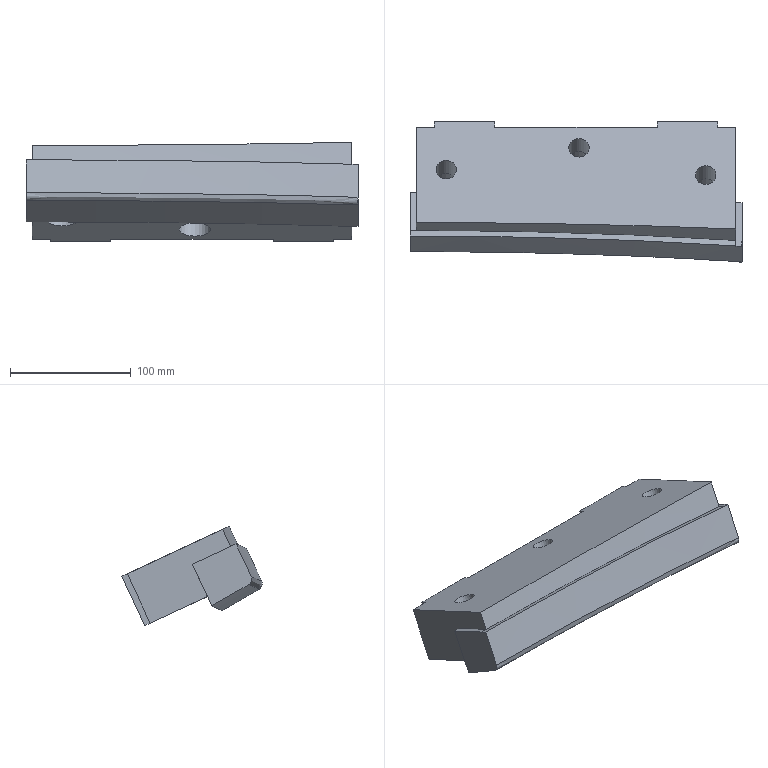Part | NX | features solid 2 | 1 solid | 33 faces | box 275 x 116.336 x 82.23 mm | volume 1182623 mm3 | plane 20 | spline 7 | cylinder 6 | commonest cylinder face diameters 17 x3 26 x3
STEP:
#1=CARTESIAN_POINT('',(270.,601.451,-143.671));
#2=VERTEX_POINT('',#1);
#3=CARTESIAN_POINT('',(255.,601.451,-143.671));
#4=VERTEX_POINT('',#3);
#5=CARTESIAN_POINT('',(575.,601.451,-143.671));
#6=DIRECTION('',(-1.,0.,0.));
#7=VECTOR('',#6,1000.);
#8=LINE('',#5,#7);
#9=EDGE_CURVE('',#2,#4,#8,.T.);
#10=ORIENTED_EDGE('',*,*,#9,.T.);
#11=CARTESIAN_POINT('',(255.,620.468,-102.887));
#12=VERTEX_POINT('',#11);
#13=CARTESIAN_POINT('',(255.,620.468,-102.887));
#14=DIRECTION('',(0.,-0.4226,-0.9063));
#15=VECTOR('',#14,1000.);
#16=LINE('',#13,#15);
#17=EDGE_CURVE('',#12,#4,#16,.T.);
#18=ORIENTED_EDGE('',*,*,#17,.F.);
#19=CARTESIAN_POINT('',(270.,620.468,-102.887));
#20=VERTEX_POINT('',#19);
#21=CARTESIAN_POINT('',(575.,620.468,-102.887));
#22=DIRECTION('',(1.,0.,0.));
#23=VECTOR('',#22,1000.);
#24=LINE('',#21,#23);
#25=EDGE_CURVE('',#20,#12,#24,.F.);
#26=ORIENTED_EDGE('',*,*,#25,.F.);
#27=CARTESIAN_POINT('',(270.,624.528,-94.181));
#28=DIRECTION('',(0.,-0.4226,-0.9063));
#29=VECTOR('',#28,1000.);
#30=LINE('',#27,#29);
#31=EDGE_CURVE('',#2,#20,#30,.F.);
#32=ORIENTED_EDGE('',*,*,#31,.F.);
#33=EDGE_LOOP('',(#10,#18,#26,#32));
#34=FACE_BOUND('',#33,.T.);
#35=CARTESIAN_POINT('',(575.,624.528,-94.181));
#36=DIRECTION('',(0.,-0.9063,0.4226));
#37=DIRECTION('',(0.,-0.4226,-0.9063));
#38=AXIS2_PLACEMENT_3D('',#35,#36,#37);
#39=PLANE('',#38);
#40=ADVANCED_FACE('',(#34),#39,.F.);
#41=CARTESIAN_POINT('',(205.,620.468,-102.887));
#42=VERTEX_POINT('',#41);
#43=CARTESIAN_POINT('',(70.,620.468,-102.887));
#44=VERTEX_POINT('',#43);
#45=CARTESIAN_POINT('',(575.,620.468,-102.887));
#46=DIRECTION('',(1.,0.,0.));
#47=VECTOR('',#46,1000.);
#48=LINE('',#45,#47);
#49=EDGE_CURVE('',#42,#44,#48,.F.);
#50=ORIENTED_EDGE('',*,*,#49,.F.);
#51=CARTESIAN_POINT('',(205.,601.451,-143.671));
#52=VERTEX_POINT('',#51);
#53=CARTESIAN_POINT('',(205.,620.468,-102.887));
#54=DIRECTION('',(0.,-0.4226,-0.9063));
#55=VECTOR('',#54,1000.);
#56=LINE('',#53,#55);
#57=EDGE_CURVE('',#42,#52,#56,.T.);
#58=ORIENTED_EDGE('',*,*,#57,.T.);
#59=CARTESIAN_POINT('',(70.,601.451,-143.671));
#60=VERTEX_POINT('',#59);
#61=CARTESIAN_POINT('',(575.,601.451,-143.671));
#62=DIRECTION('',(-1.,0.,0.));
#63=VECTOR('',#62,1000.);
#64=LINE('',#61,#63);
#65=EDGE_CURVE('',#52,#60,#64,.T.);
#66=ORIENTED_EDGE('',*,*,#65,.T.);
#67=CARTESIAN_POINT('',(70.,620.468,-102.887));
#68=DIRECTION('',(0.,-0.4226,-0.9063));
#69=VECTOR('',#68,1000.);
#70=LINE('',#67,#69);
#71=EDGE_CURVE('',#44,#60,#70,.T.);
#72=ORIENTED_EDGE('',*,*,#71,.F.);
#73=EDGE_LOOP('',(#50,#58,#66,#72));
#74=FACE_BOUND('',#73,.T.);
#75=CARTESIAN_POINT('',(575.,624.528,-94.181));
#76=DIRECTION('',(0.,-0.9063,0.4226));
#77=DIRECTION('',(0.,-0.4226,-0.9063));
#78=AXIS2_PLACEMENT_3D('',#75,#76,#77);
#79=PLANE('',#78);
#80=ADVANCED_FACE('',(#74),#79,.F.);
#81=CARTESIAN_POINT('',(20.,620.468,-102.887));
#82=VERTEX_POINT('',#81);
#83=CARTESIAN_POINT('',(5.,620.468,-102.887));
#84=VERTEX_POINT('',#83);
#85=CARTESIAN_POINT('',(575.,620.468,-102.887));
#86=DIRECTION('',(1.,0.,0.));
#87=VECTOR('',#86,1000.);
#88=LINE('',#85,#87);
#89=EDGE_CURVE('',#82,#84,#88,.F.);
#90=ORIENTED_EDGE('',*,*,#89,.F.);
#91=CARTESIAN_POINT('',(20.,601.451,-143.671));
#92=VERTEX_POINT('',#91);
#93=CARTESIAN_POINT('',(20.,620.468,-102.887));
#94=DIRECTION('',(0.,-0.4226,-0.9063));
#95=VECTOR('',#94,1000.);
#96=LINE('',#93,#95);
#97=EDGE_CURVE('',#82,#92,#96,.T.);
#98=ORIENTED_EDGE('',*,*,#97,.T.);
#99=CARTESIAN_POINT('',(5.,601.451,-143.671));
#100=VERTEX_POINT('',#99);
#101=CARTESIAN_POINT('',(575.,601.451,-143.671));
#102=DIRECTION('',(-1.,0.,0.));
#103=VECTOR('',#102,1000.);
#104=LINE('',#101,#103);
#105=EDGE_CURVE('',#92,#100,#104,.T.);
#106=ORIENTED_EDGE('',*,*,#105,.T.);
#107=CARTESIAN_POINT('',(5.,624.528,-94.181));
#108=DIRECTION('',(0.,0.4226,0.9063));
#109=VECTOR('',#108,1000.);
#110=LINE('',#107,#109);
#111=EDGE_CURVE('',#84,#100,#110,.F.);
#112=ORIENTED_EDGE('',*,*,#111,.F.);
#113=EDGE_LOOP('',(#90,#98,#106,#112));
#114=FACE_BOUND('',#113,.T.);
#115=CARTESIAN_POINT('',(575.,624.528,-94.181));
#116=DIRECTION('',(0.,-0.9063,0.4226));
#117=DIRECTION('',(0.,-0.4226,-0.9063));
#118=AXIS2_PLACEMENT_3D('',#115,#116,#117);
#119=PLANE('',#118);
#120=ADVANCED_FACE('',(#114),#119,.F.);
#121=CARTESIAN_POINT('',(275.,521.829,-81.79));
#122=VERTEX_POINT('',#121);
#123=CARTESIAN_POINT('',(275.,526.352,-83.884));
#124=VERTEX_POINT('',#123);
#125=CARTESIAN_POINT('',(275.,521.829,-81.79));
#126=CARTESIAN_POINT('',(275.,523.337,-82.488));
#127=CARTESIAN_POINT('',(275.,524.845,-83.186));
#128=CARTESIAN_POINT('',(275.,526.352,-83.884));
#129=B_SPLINE_CURVE_WITH_KNOTS('',3,(#125,#126,#127,#128),.UNSPECIFIED.,.F.,.F.,(4,4),(0.001536,0.00652),.UNSPECIFIED.);
#130=EDGE_CURVE('',#122,#124,#129,.T.);
#131=ORIENTED_EDGE('',*,*,#130,.T.);
#132=CARTESIAN_POINT('',(274.761,521.845,-81.782));
#133=VERTEX_POINT('',#132);
#134=CARTESIAN_POINT('',(275.,526.352,-83.884));
#135=CARTESIAN_POINT('',(274.92,524.85,-83.183));
#136=CARTESIAN_POINT('',(274.84,523.348,-82.483));
#137=CARTESIAN_POINT('',(274.761,521.845,-81.782));
#138=B_SPLINE_CURVE_WITH_KNOTS('',3,(#134,#135,#136,#137),.UNSPECIFIED.,.F.,.F.,(4,4),(0.00005195,0.005031),.UNSPECIFIED.);
#139=EDGE_CURVE('',#124,#133,#138,.T.);
#140=ORIENTED_EDGE('',*,*,#139,.T.);
#141=CARTESIAN_POINT('',(275.,521.829,-81.79));
#142=CARTESIAN_POINT('',(274.92,521.835,-81.787));
#143=CARTESIAN_POINT('',(274.84,521.84,-81.785));
#144=CARTESIAN_POINT('',(274.761,521.845,-81.782));
#145=B_SPLINE_CURVE_WITH_KNOTS('',3,(#141,#142,#143,#144),.UNSPECIFIED.,.F.,.F.,(4,4),(0.2861,0.2864),.UNSPECIFIED.);
#146=EDGE_CURVE('',#122,#133,#145,.T.);
#147=ORIENTED_EDGE('',*,*,#146,.F.);
#148=EDGE_LOOP('',(#131,#140,#147));
#149=FACE_BOUND('',#148,.T.);
#150=CARTESIAN_POINT('',(275.243,526.363,-83.904));
#151=CARTESIAN_POINT('',(275.162,526.369,-83.901));
#152=CARTESIAN_POINT('',(275.082,526.374,-83.899));
#153=CARTESIAN_POINT('',(275.001,526.379,-83.896));
#154=CARTESIAN_POINT('',(275.242,526.355,-83.9));
#155=CARTESIAN_POINT('',(275.162,526.361,-83.898));
#156=CARTESIAN_POINT('',(275.081,526.366,-83.895));
#157=CARTESIAN_POINT('',(275.001,526.372,-83.893));
#158=CARTESIAN_POINT('',(275.,521.802,-81.777));
#159=CARTESIAN_POINT('',(274.92,521.808,-81.775));
#160=CARTESIAN_POINT('',(274.839,521.813,-81.772));
#161=CARTESIAN_POINT('',(274.759,521.818,-81.77));
#162=B_SPLINE_SURFACE_WITH_KNOTS('',1,3,((#150,#151,#152,#153),(#154,#155,#156,#157),(#158,#159,#160,#161)),.RULED_SURF.,.F.,.F.,.F.,(2,1,2),(4,4),(-0.0008614,0.,0.503),(0.2539,0.2541),.PIECEWISE_BEZIER_KNOTS.);
#163=ADVANCED_FACE('',(#149),#162,.F.);
#164=CARTESIAN_POINT('',(0.,566.489,-94.945));
#165=VERTEX_POINT('',#164);
#166=CARTESIAN_POINT('',(0.,534.859,-80.196));
#167=VERTEX_POINT('',#166);
#168=CARTESIAN_POINT('',(0.,-410.961,360.847));
#169=DIRECTION('',(0.,-0.9063,0.4226));
#170=VECTOR('',#169,1000.);
#171=LINE('',#168,#170);
#172=EDGE_CURVE('',#165,#167,#171,.T.);
#173=ORIENTED_EDGE('',*,*,#172,.F.);
#174=CARTESIAN_POINT('',(0.1494,550.411,-129.426));
#175=VERTEX_POINT('',#174);
#176=CARTESIAN_POINT('',(0.,541.565,-148.396));
#177=DIRECTION('',(0.,0.4226,0.9063));
#178=VECTOR('',#177,1000.);
#179=LINE('',#176,#178);
#180=EDGE_CURVE('',#175,#165,#179,.T.);
#181=ORIENTED_EDGE('',*,*,#180,.F.);
#182=CARTESIAN_POINT('',(0.1308,519.6,-111.637));
#183=VERTEX_POINT('',#182);
#184=CARTESIAN_POINT('',(0.,519.507,-111.584));
#185=CARTESIAN_POINT('',(0.,529.898,-117.583));
#186=CARTESIAN_POINT('',(0.,540.289,-123.583));
#187=CARTESIAN_POINT('',(0.,550.68,-129.582));
#188=B_SPLINE_CURVE_WITH_KNOTS('',3,(#184,#185,#186,#187),.UNSPECIFIED.,.F.,.F.,(4,4),(0.,1.),.UNSPECIFIED.);
#189=EDGE_CURVE('',#183,#175,#188,.T.);
#190=ORIENTED_EDGE('',*,*,#189,.F.);
#191=CARTESIAN_POINT('',(0.1262,517.66,-105.247));
#192=VERTEX_POINT('',#191);
#193=CARTESIAN_POINT('',(0.,517.66,-105.248));
#194=CARTESIAN_POINT('',(0.,517.387,-105.835));
#195=CARTESIAN_POINT('',(0.,517.07,-107.013));
#196=CARTESIAN_POINT('',(0.,517.318,-108.896));
#197=CARTESIAN_POINT('',(0.,518.194,-110.583));
#198=CARTESIAN_POINT('',(0.,519.13,-111.367));
#199=CARTESIAN_POINT('',(0.,519.692,-111.691));
#200=B_SPLINE_CURVE_WITH_KNOTS('',3,(#193,#194,#195,#196,#197,#198,#199),.UNSPECIFIED.,.F.,.F.,(4,1,1,1,4),(0.,0.25,0.5,0.75,1.),.UNSPECIFIED.);
#201=EDGE_CURVE('',#192,#183,#200,.T.);
#202=ORIENTED_EDGE('',*,*,#201,.F.);
#203=CARTESIAN_POINT('',(0.,530.327,-78.083));
#204=VERTEX_POINT('',#203);
#205=CARTESIAN_POINT('',(0.,514.598,-111.815));
#206=DIRECTION('',(0.,0.4226,0.9063));
#207=VECTOR('',#206,1000.);
#208=LINE('',#205,#207);
#209=EDGE_CURVE('',#192,#204,#208,.T.);
#210=ORIENTED_EDGE('',*,*,#209,.T.);
#211=CARTESIAN_POINT('',(0.,530.327,-78.083));
#212=CARTESIAN_POINT('',(0.,531.838,-78.787));
#213=CARTESIAN_POINT('',(0.,533.349,-79.492));
#214=CARTESIAN_POINT('',(0.,534.859,-80.196));
#215=B_SPLINE_CURVE_WITH_KNOTS('',3,(#211,#212,#213,#214),.UNSPECIFIED.,.F.,.F.,(4,4),(0.001534,0.006534),.UNSPECIFIED.);
#216=EDGE_CURVE('',#204,#167,#215,.T.);
#217=ORIENTED_EDGE('',*,*,#216,.T.);
#218=EDGE_LOOP('',(#173,#181,#190,#202,#210,#217));
#219=FACE_BOUND('',#218,.T.);
#220=CARTESIAN_POINT('',(0.,-402.415,379.173));
#221=DIRECTION('',(-1.,0.,0.));
#222=DIRECTION('',(0.,-1.,0.));
#223=AXIS2_PLACEMENT_3D('',#220,#221,#222);
#224=PLANE('',#223);
#225=ADVANCED_FACE('',(#219),#224,.T.);
#226=CARTESIAN_POINT('',(275.,541.913,-133.245));
#227=VERTEX_POINT('',#226);
#228=CARTESIAN_POINT('',(275.,558.04,-98.66));
#229=VERTEX_POINT('',#228);
#230=CARTESIAN_POINT('',(275.,536.047,-145.824));
#231=DIRECTION('',(0.,0.4226,0.9063));
#232=VECTOR('',#231,1000.);
#233=LINE('',#230,#232);
#234=EDGE_CURVE('',#227,#229,#233,.T.);
#235=ORIENTED_EDGE('',*,*,#234,.T.);
#236=CARTESIAN_POINT('',(275.,-413.893,354.56));
#237=DIRECTION('',(0.,-0.9063,0.4226));
#238=VECTOR('',#237,1000.);
#239=LINE('',#236,#238);
#240=EDGE_CURVE('',#229,#124,#239,.T.);
#241=ORIENTED_EDGE('',*,*,#240,.T.);
#242=ORIENTED_EDGE('',*,*,#130,.F.);
#243=CARTESIAN_POINT('',(275.,509.13,-109.022));
#244=VERTEX_POINT('',#243);
#245=CARTESIAN_POINT('',(275.,509.037,-109.222));
#246=DIRECTION('',(0.,0.4226,0.9063));
#247=VECTOR('',#246,1000.);
#248=LINE('',#245,#247);
#249=EDGE_CURVE('',#244,#122,#248,.T.);
#250=ORIENTED_EDGE('',*,*,#249,.F.);
#251=CARTESIAN_POINT('',(275.,511.154,-115.455));
#252=VERTEX_POINT('',#251);
#253=CARTESIAN_POINT('',(275.,509.13,-109.022));
#254=CARTESIAN_POINT('',(275.,508.604,-110.151));
#255=CARTESIAN_POINT('',(275.,508.441,-112.771));
#256=CARTESIAN_POINT('',(275.,510.076,-114.832));
#257=CARTESIAN_POINT('',(275.,511.154,-115.455));
#258=B_SPLINE_CURVE_WITH_KNOTS('',3,(#253,#254,#255,#256,#257),.UNSPECIFIED.,.F.,.F.,(4,1,4),(0.,0.003682,0.007364),.UNSPECIFIED.);
#259=EDGE_CURVE('',#244,#252,#258,.T.);
#260=ORIENTED_EDGE('',*,*,#259,.T.);
#261=CARTESIAN_POINT('',(275.,511.154,-115.455));
#262=CARTESIAN_POINT('',(275.,521.407,-121.385));
#263=CARTESIAN_POINT('',(275.,531.66,-127.315));
#264=CARTESIAN_POINT('',(275.,541.913,-133.245));
#265=B_SPLINE_CURVE_WITH_KNOTS('',3,(#261,#262,#263,#264),.UNSPECIFIED.,.F.,.F.,(4,4),(0.0002564,0.03579),.UNSPECIFIED.);
#266=EDGE_CURVE('',#252,#227,#265,.T.);
#267=ORIENTED_EDGE('',*,*,#266,.T.);
#268=EDGE_LOOP('',(#235,#241,#242,#250,#260,#267));
#269=FACE_BOUND('',#268,.T.);
#270=CARTESIAN_POINT('',(275.,-402.415,379.173));
#271=DIRECTION('',(-1.,0.,0.));
#272=DIRECTION('',(0.,-1.,0.));
#273=AXIS2_PLACEMENT_3D('',#270,#271,#272);
#274=PLANE('',#273);
#275=ADVANCED_FACE('',(#269),#274,.F.);
#276=CARTESIAN_POINT('',(30.,593.005,-90.081));
#277=VERTEX_POINT('',#276);
#278=CARTESIAN_POINT('',(30.,585.302,-86.488));
#279=DIRECTION('',(0.,-0.4226,-0.9063));
#280=DIRECTION('',(0.,0.9063,-0.4226));
#281=AXIS2_PLACEMENT_3D('',#278,#279,#280);
#282=CIRCLE('',#281,8.5);
#283=EDGE_CURVE('',#277,#277,#282,.T.);
#284=ORIENTED_EDGE('',*,*,#283,.T.);
#285=EDGE_LOOP('',(#284));
#286=FACE_BOUND('',#285,.T.);
#287=CARTESIAN_POINT('',(140.,611.132,-98.533));
#288=VERTEX_POINT('',#287);
#289=CARTESIAN_POINT('',(140.,603.428,-94.941));
#290=DIRECTION('',(0.,-0.4226,-0.9063));
#291=DIRECTION('',(0.,0.9063,-0.4226));
#292=AXIS2_PLACEMENT_3D('',#289,#290,#291);
#293=CIRCLE('',#292,8.5);
#294=EDGE_CURVE('',#288,#288,#293,.T.);
#295=ORIENTED_EDGE('',*,*,#294,.T.);
#296=EDGE_LOOP('',(#295));
#297=FACE_BOUND('',#296,.T.);
#298=CARTESIAN_POINT('',(245.,588.474,-87.968));
#299=VERTEX_POINT('',#298);
#300=CARTESIAN_POINT('',(245.,580.77,-84.375));
#301=DIRECTION('',(0.,-0.4226,-0.9063));
#302=DIRECTION('',(0.,0.9063,-0.4226));
#303=AXIS2_PLACEMENT_3D('',#300,#301,#302);
#304=CIRCLE('',#303,8.5);
#305=EDGE_CURVE('',#299,#299,#304,.T.);
#306=ORIENTED_EDGE('',*,*,#305,.T.);
#307=EDGE_LOOP('',(#306));
#308=FACE_BOUND('',#307,.T.);
#309=ORIENTED_EDGE('',*,*,#25,.T.);
#310=CARTESIAN_POINT('',(255.,625.,-105.));
#311=VERTEX_POINT('',#310);
#312=CARTESIAN_POINT('',(255.,620.468,-102.887));
#313=DIRECTION('',(0.,-0.9063,0.4226));
#314=VECTOR('',#313,1000.);
#315=LINE('',#312,#314);
#316=EDGE_CURVE('',#12,#311,#315,.F.);
#317=ORIENTED_EDGE('',*,*,#316,.T.);
#318=CARTESIAN_POINT('',(205.,625.,-105.));
#319=VERTEX_POINT('',#318);
#320=CARTESIAN_POINT('',(255.,625.,-105.));
#321=DIRECTION('',(1.,0.,0.));
#322=VECTOR('',#321,1000.);
#323=LINE('',#320,#322);
#324=EDGE_CURVE('',#311,#319,#323,.F.);
#325=ORIENTED_EDGE('',*,*,#324,.T.);
#326=CARTESIAN_POINT('',(205.,620.468,-102.887));
#327=DIRECTION('',(0.,-0.9063,0.4226));
#328=VECTOR('',#327,1000.);
#329=LINE('',#326,#328);
#330=EDGE_CURVE('',#42,#319,#329,.F.);
#331=ORIENTED_EDGE('',*,*,#330,.F.);
#332=ORIENTED_EDGE('',*,*,#49,.T.);
#333=CARTESIAN_POINT('',(70.,625.,-105.));
#334=VERTEX_POINT('',#333);
#335=CARTESIAN_POINT('',(70.,620.468,-102.887));
#336=DIRECTION('',(0.,-0.9063,0.4226));
#337=VECTOR('',#336,1000.);
#338=LINE('',#335,#337);
#339=EDGE_CURVE('',#44,#334,#338,.F.);
#340=ORIENTED_EDGE('',*,*,#339,.T.);
#341=CARTESIAN_POINT('',(20.,625.,-105.));
#342=VERTEX_POINT('',#341);
#343=CARTESIAN_POINT('',(20.,625.,-105.));
#344=DIRECTION('',(1.,0.,0.));
#345=VECTOR('',#344,1000.);
#346=LINE('',#343,#345);
#347=EDGE_CURVE('',#342,#334,#346,.T.);
#348=ORIENTED_EDGE('',*,*,#347,.F.);
#349=CARTESIAN_POINT('',(20.,620.468,-102.887));
#350=DIRECTION('',(0.,-0.9063,0.4226));
#351=VECTOR('',#350,1000.);
#352=LINE('',#349,#351);
#353=EDGE_CURVE('',#82,#342,#352,.F.);
#354=ORIENTED_EDGE('',*,*,#353,.F.);
#355=ORIENTED_EDGE('',*,*,#89,.T.);
#356=CARTESIAN_POINT('',(5.,541.457,-66.043));
#357=VERTEX_POINT('',#356);
#358=CARTESIAN_POINT('',(5.,568.557,-78.68));
#359=DIRECTION('',(0.,-0.9063,0.4226));
#360=VECTOR('',#359,1000.);
#361=LINE('',#358,#360);
#362=EDGE_CURVE('',#84,#357,#361,.T.);
#363=ORIENTED_EDGE('',*,*,#362,.T.);
#364=CARTESIAN_POINT('',(270.,536.118,-63.554));
#365=VERTEX_POINT('',#364);
#366=CARTESIAN_POINT('',(5.,541.457,-66.043));
#367=CARTESIAN_POINT('',(49.188,541.427,-66.029));
#368=CARTESIAN_POINT('',(137.544,540.561,-65.626));
#369=CARTESIAN_POINT('',(225.858,537.997,-64.43));
#370=CARTESIAN_POINT('',(270.,536.118,-63.554));
#371=B_SPLINE_CURVE_WITH_KNOTS('',3,(#366,#367,#368,#369,#370),.UNSPECIFIED.,.F.,.F.,(4,1,4),(0.,0.1325,0.2651),.UNSPECIFIED.);
#372=EDGE_CURVE('',#357,#365,#371,.T.);
#373=ORIENTED_EDGE('',*,*,#372,.T.);
#374=CARTESIAN_POINT('',(270.,568.557,-78.68));
#375=DIRECTION('',(0.,0.9063,-0.4226));
#376=VECTOR('',#375,1000.);
#377=LINE('',#374,#376);
#378=EDGE_CURVE('',#365,#20,#377,.T.);
#379=ORIENTED_EDGE('',*,*,#378,.T.);
#380=EDGE_LOOP('',(#309,#317,#325,#331,#332,#340,#348,#354,#355,#363,#373,#379));
#381=FACE_BOUND('',#380,.T.);
#382=CARTESIAN_POINT('',(0.0001507,568.557,-78.68));
#383=DIRECTION('',(0.,-0.4226,-0.9063));
#384=DIRECTION('',(0.,0.9063,-0.4226));
#385=AXIS2_PLACEMENT_3D('',#382,#383,#384);
#386=PLANE('',#385);
#387=ADVANCED_FACE('',(#286,#297,#308,#381),#386,.F.);
#388=CARTESIAN_POINT('',(275.,541.913,-133.245));
#389=CARTESIAN_POINT('',(252.161,543.463,-132.522));
#390=CARTESIAN_POINT('',(206.445,546.02,-131.369));
#391=CARTESIAN_POINT('',(137.772,548.579,-130.204));
#392=CARTESIAN_POINT('',(69.042,550.086,-129.551));
#393=CARTESIAN_POINT('',(23.212,550.391,-129.464));
#394=CARTESIAN_POINT('',(0.2987,550.41,-129.427));
#395=B_SPLINE_CURVE_WITH_KNOTS('',3,(#388,#389,#390,#391,#392,#393,#394),.UNSPECIFIED.,.F.,.F.,(4,1,1,1,4),(0.3277,0.3968,0.4659,0.535,0.6041),.UNSPECIFIED.);
#396=EDGE_CURVE('',#227,#175,#395,.T.);
#397=ORIENTED_EDGE('',*,*,#396,.T.);
#398=ORIENTED_EDGE('',*,*,#180,.T.);
#399=CARTESIAN_POINT('',(5.,566.487,-94.945));
#400=VERTEX_POINT('',#399);
#401=CARTESIAN_POINT('',(5.,566.487,-94.945));
#402=CARTESIAN_POINT('',(3.333,566.489,-94.945));
#403=CARTESIAN_POINT('',(1.667,566.489,-94.945));
#404=CARTESIAN_POINT('',(0.,566.489,-94.945));
#405=B_SPLINE_CURVE_WITH_KNOTS('',3,(#401,#402,#403,#404),.UNSPECIFIED.,.F.,.F.,(4,4),(0.,0.005),.UNSPECIFIED.);
#406=EDGE_CURVE('',#400,#165,#405,.T.);
#407=ORIENTED_EDGE('',*,*,#406,.F.);
#408=CARTESIAN_POINT('',(5.,554.069,-121.576));
#409=VERTEX_POINT('',#408);
#410=CARTESIAN_POINT('',(5.,587.618,-49.629));
#411=DIRECTION('',(0.,0.4226,0.9063));
#412=VECTOR('',#411,1000.);
#413=LINE('',#410,#412);
#414=EDGE_CURVE('',#409,#400,#413,.T.);
#415=ORIENTED_EDGE('',*,*,#414,.F.);
#416=CARTESIAN_POINT('',(270.,548.769,-119.105));
#417=VERTEX_POINT('',#416);
#418=CARTESIAN_POINT('',(270.,548.769,-119.105));
#419=CARTESIAN_POINT('',(225.874,550.647,-119.981));
#420=CARTESIAN_POINT('',(137.542,553.172,-121.158));
#421=CARTESIAN_POINT('',(49.177,554.039,-121.562));
#422=CARTESIAN_POINT('',(5.,554.069,-121.576));
#423=B_SPLINE_CURVE_WITH_KNOTS('',3,(#418,#419,#420,#421,#422),.UNSPECIFIED.,.F.,.F.,(4,1,4),(0.3304,0.4638,0.5972),.UNSPECIFIED.);
#424=EDGE_CURVE('',#409,#417,#423,.F.);
#425=ORIENTED_EDGE('',*,*,#424,.T.);
#426=CARTESIAN_POINT('',(270.,558.255,-98.76));
#427=VERTEX_POINT('',#426);
#428=CARTESIAN_POINT('',(270.,579.386,-53.445));
#429=DIRECTION('',(0.,0.4226,0.9063));
#430=VECTOR('',#429,1000.);
#431=LINE('',#428,#430);
#432=EDGE_CURVE('',#417,#427,#431,.T.);
#433=ORIENTED_EDGE('',*,*,#432,.T.);
#434=CARTESIAN_POINT('',(275.,558.04,-98.66));
#435=CARTESIAN_POINT('',(273.333,558.113,-98.694));
#436=CARTESIAN_POINT('',(271.667,558.185,-98.727));
#437=CARTESIAN_POINT('',(270.,558.255,-98.76));
#438=B_SPLINE_CURVE_WITH_KNOTS('',3,(#434,#435,#436,#437),.UNSPECIFIED.,.F.,.F.,(4,4),(0.,0.005006),.UNSPECIFIED.);
#439=EDGE_CURVE('',#229,#427,#438,.T.);
#440=ORIENTED_EDGE('',*,*,#439,.F.);
#441=ORIENTED_EDGE('',*,*,#234,.F.);
#442=EDGE_LOOP('',(#397,#398,#407,#415,#425,#433,#440,#441));
#443=FACE_BOUND('',#442,.T.);
#444=CARTESIAN_POINT('',(275.,541.798,-133.491));
#445=CARTESIAN_POINT('',(275.,560.972,-92.373));
#446=CARTESIAN_POINT('',(229.14,543.799,-134.424));
#447=CARTESIAN_POINT('',(229.14,562.973,-93.306));
#448=CARTESIAN_POINT('',(137.488,546.449,-135.659));
#449=CARTESIAN_POINT('',(137.488,565.622,-94.541));
#450=CARTESIAN_POINT('',(45.83,547.315,-136.063));
#451=CARTESIAN_POINT('',(45.83,566.489,-94.945));
#452=CARTESIAN_POINT('',(0.,547.316,-136.063));
#453=CARTESIAN_POINT('',(0.,566.489,-94.945));
#454=B_SPLINE_SURFACE_WITH_KNOTS('',3,1,((#444,#445),(#446,#447),(#448,#449),(#450,#451),(#452,#453)),.SURF_OF_LINEAR_EXTRUSION.,.F.,.F.,.F.,(4,1,4),(2,2),(0.259,0.3795,0.5),(0.,1.),.UNSPECIFIED.);
#455=ADVANCED_FACE('',(#443),#454,.T.);
#456=ORIENTED_EDGE('',*,*,#266,.F.);
#457=CARTESIAN_POINT('',(275.,511.154,-115.455));
#458=CARTESIAN_POINT('',(252.136,512.708,-114.74));
#459=CARTESIAN_POINT('',(206.371,515.266,-113.597));
#460=CARTESIAN_POINT('',(137.64,517.859,-112.459));
#461=CARTESIAN_POINT('',(68.827,519.374,-111.816));
#462=CARTESIAN_POINT('',(22.943,519.674,-111.729));
#463=CARTESIAN_POINT('',(0.00009814,519.692,-111.691));
#464=B_SPLINE_CURVE_WITH_KNOTS('',3,(#457,#458,#459,#460,#461,#462,#463),.UNSPECIFIED.,.F.,.F.,(4,1,1,1,4),(0.08355,0.1523,0.2211,0.2899,0.3587),.UNSPECIFIED.);
#465=EDGE_CURVE('',#252,#183,#464,.T.);
#466=ORIENTED_EDGE('',*,*,#465,.T.);
#467=ORIENTED_EDGE('',*,*,#189,.T.);
#468=ORIENTED_EDGE('',*,*,#396,.F.);
#469=EDGE_LOOP('',(#456,#466,#467,#468));
#470=FACE_BOUND('',#469,.T.);
#471=CARTESIAN_POINT('',(277.219,510.812,-115.416));
#472=CARTESIAN_POINT('',(276.64,541.986,-133.405));
#473=CARTESIAN_POINT('',(264.567,511.676,-115.01));
#474=CARTESIAN_POINT('',(264.035,542.849,-133.001));
#475=CARTESIAN_POINT('',(250.894,512.514,-114.625));
#476=CARTESIAN_POINT('',(250.405,543.687,-132.617));
#477=CARTESIAN_POINT('',(218.319,514.321,-113.806));
#478=CARTESIAN_POINT('',(217.92,545.495,-131.799));
#479=CARTESIAN_POINT('',(197.638,515.298,-113.372));
#480=CARTESIAN_POINT('',(197.285,546.471,-131.367));
#481=CARTESIAN_POINT('',(158.795,516.84,-112.697));
#482=CARTESIAN_POINT('',(158.522,548.013,-130.693));
#483=CARTESIAN_POINT('',(138.351,517.497,-112.414));
#484=CARTESIAN_POINT('',(138.119,548.671,-130.411));
#485=CARTESIAN_POINT('',(99.232,518.495,-111.988));
#486=CARTESIAN_POINT('',(99.076,549.669,-129.985));
#487=CARTESIAN_POINT('',(79.034,518.875,-111.827));
#488=CARTESIAN_POINT('',(78.917,550.049,-129.825));
#489=CARTESIAN_POINT('',(39.648,519.364,-111.64));
#490=CARTESIAN_POINT('',(39.596,550.537,-129.638));
#491=CARTESIAN_POINT('',(19.699,519.481,-111.61));
#492=CARTESIAN_POINT('',(19.673,550.655,-129.608));
#493=CARTESIAN_POINT('',(-0.5516,519.508,-111.583));
#494=CARTESIAN_POINT('',(-0.5754,550.681,-129.581));
#495=CARTESIAN_POINT('',(-1.103,519.509,-111.583));
#496=CARTESIAN_POINT('',(-1.127,550.682,-129.581));
#497=CARTESIAN_POINT('',(-1.655,519.509,-111.582));
#498=CARTESIAN_POINT('',(-1.679,550.683,-129.58));
#499=B_SPLINE_SURFACE_WITH_KNOTS('',3,1,((#471,#472),(#473,#474),(#475,#476),(#477,#478),(#479,#480),(#481,#482),(#483,#484),(#485,#486),(#487,#488),(#489,#490),(#491,#492),(#493,#494),(#495,#496),(#497,#498)),.RULED_SURF.,.F.,.F.,.F.,(4,1,1,1,1,1,1,1,1,2,4),(2,2),(0.3232,0.3929,0.3985,0.5026,0.5067,0.6122,0.615,0.7219,0.7233,0.8315,0.8346),(0.1701,0.9376),.UNSPECIFIED.);
#500=ADVANCED_FACE('',(#470),#499,.T.);
#501=ORIENTED_EDGE('',*,*,#146,.T.);
#502=CARTESIAN_POINT('',(270.,522.051,-81.878));
#503=VERTEX_POINT('',#502);
#504=CARTESIAN_POINT('',(274.761,521.845,-81.782));
#505=CARTESIAN_POINT('',(273.174,521.915,-81.814));
#506=CARTESIAN_POINT('',(271.587,521.983,-81.846));
#507=CARTESIAN_POINT('',(270.,522.051,-81.878));
#508=B_SPLINE_CURVE_WITH_KNOTS('',3,(#504,#505,#506,#507),.UNSPECIFIED.,.F.,.F.,(4,4),(0.0002397,0.005006),.UNSPECIFIED.);
#509=EDGE_CURVE('',#133,#503,#508,.T.);
#510=ORIENTED_EDGE('',*,*,#509,.T.);
#511=CARTESIAN_POINT('',(270.,522.164,-81.636));
#512=VERTEX_POINT('',#511);
#513=CARTESIAN_POINT('',(270.,517.164,-92.357));
#514=DIRECTION('',(0.,0.4226,0.9063));
#515=VECTOR('',#514,1000.);
#516=LINE('',#513,#515);
#517=EDGE_CURVE('',#503,#512,#516,.T.);
#518=ORIENTED_EDGE('',*,*,#517,.T.);
#519=CARTESIAN_POINT('',(270.,522.164,-81.636));
#520=CARTESIAN_POINT('',(225.085,525.129,-80.275));
#521=CARTESIAN_POINT('',(135.102,529.088,-78.555));
#522=CARTESIAN_POINT('',(45.034,530.328,-78.082));
#523=CARTESIAN_POINT('',(0.,530.327,-78.083));
#524=B_SPLINE_CURVE_WITH_KNOTS('',3,(#519,#520,#521,#522,#523),.UNSPECIFIED.,.F.,.F.,(4,1,4),(0.2911,0.4249,0.5587),.UNSPECIFIED.);
#525=EDGE_CURVE('',#512,#204,#524,.T.);
#526=ORIENTED_EDGE('',*,*,#525,.T.);
#527=ORIENTED_EDGE('',*,*,#209,.F.);
#528=CARTESIAN_POINT('',(0.2523,517.66,-105.248));
#529=CARTESIAN_POINT('',(23.175,517.642,-105.286));
#530=CARTESIAN_POINT('',(69.016,517.339,-105.374));
#531=CARTESIAN_POINT('',(137.766,515.824,-106.019));
#532=CARTESIAN_POINT('',(206.433,513.234,-107.159));
#533=CARTESIAN_POINT('',(252.157,510.681,-108.306));
#534=CARTESIAN_POINT('',(275.,509.13,-109.022));
#535=B_SPLINE_CURVE_WITH_KNOTS('',3,(#528,#529,#530,#531,#532,#533,#534),.UNSPECIFIED.,.F.,.F.,(4,1,1,1,4),(0.,0.06876,0.1375,0.2063,0.2751),.UNSPECIFIED.);
#536=EDGE_CURVE('',#192,#244,#535,.T.);
#537=ORIENTED_EDGE('',*,*,#536,.T.);
#538=ORIENTED_EDGE('',*,*,#249,.T.);
#539=EDGE_LOOP('',(#501,#510,#518,#526,#527,#537,#538));
#540=FACE_BOUND('',#539,.T.);
#541=CARTESIAN_POINT('',(275.,509.036,-109.224));
#542=CARTESIAN_POINT('',(275.,524.861,-75.289));
#543=CARTESIAN_POINT('',(229.257,511.037,-110.156));
#544=CARTESIAN_POINT('',(229.257,526.861,-76.221));
#545=CARTESIAN_POINT('',(137.607,513.728,-111.411));
#546=CARTESIAN_POINT('',(137.607,529.552,-77.476));
#547=CARTESIAN_POINT('',(45.87,514.597,-111.817));
#548=CARTESIAN_POINT('',(45.87,530.421,-77.882));
#549=CARTESIAN_POINT('',(0.,514.597,-111.817));
#550=CARTESIAN_POINT('',(0.,530.421,-77.882));
#551=B_SPLINE_SURFACE_WITH_KNOTS('',3,1,((#541,#542),(#543,#544),(#545,#546),(#547,#548),(#549,#550)),.SURF_OF_LINEAR_EXTRUSION.,.F.,.F.,.F.,(4,1,4),(2,2),(0.2561,0.3781,0.5),(0.,1.),.UNSPECIFIED.);
#552=ADVANCED_FACE('',(#540),#551,.F.);
#553=ORIENTED_EDGE('',*,*,#259,.F.);
#554=ORIENTED_EDGE('',*,*,#536,.F.);
#555=ORIENTED_EDGE('',*,*,#201,.T.);
#556=ORIENTED_EDGE('',*,*,#465,.F.);
#557=EDGE_LOOP('',(#553,#554,#555,#556));
#558=FACE_BOUND('',#557,.T.);
#559=CARTESIAN_POINT('',(-1.654,519.693,-111.688));
#560=CARTESIAN_POINT('',(-1.652,515.725,-109.397));
#561=CARTESIAN_POINT('',(-1.644,517.661,-105.245));
#562=CARTESIAN_POINT('',(21.595,519.68,-111.729));
#563=CARTESIAN_POINT('',(21.581,515.712,-109.438));
#564=CARTESIAN_POINT('',(21.588,517.649,-105.286));
#565=CARTESIAN_POINT('',(68.038,519.39,-111.808));
#566=CARTESIAN_POINT('',(67.992,515.422,-109.517));
#567=CARTESIAN_POINT('',(68.049,517.358,-105.365));
#568=CARTESIAN_POINT('',(137.705,517.861,-112.458));
#569=CARTESIAN_POINT('',(137.609,513.898,-110.167));
#570=CARTESIAN_POINT('',(137.725,515.83,-106.017));
#571=CARTESIAN_POINT('',(207.272,515.229,-113.613));
#572=CARTESIAN_POINT('',(207.124,511.272,-111.321));
#573=CARTESIAN_POINT('',(207.313,513.199,-107.175));
#574=CARTESIAN_POINT('',(253.589,512.623,-114.778));
#575=CARTESIAN_POINT('',(253.404,508.675,-112.484));
#576=CARTESIAN_POINT('',(253.641,510.594,-108.344));
#577=CARTESIAN_POINT('',(276.715,511.036,-115.509));
#578=CARTESIAN_POINT('',(276.518,507.094,-113.215));
#579=CARTESIAN_POINT('',(276.78,509.009,-109.079));
#580=(BOUNDED_SURFACE()B_SPLINE_SURFACE(3,2,((#559,#560,#561),(#562,#563,#564),(#565,#566,#567),(#568,#569,#570),(#571,#572,#573),(#574,#575,#576),(#577,#578,#579)),.UNSPECIFIED.,.F.,.F.,.F.)B_SPLINE_SURFACE_WITH_KNOTS((4,1,1,1,4),(3,3),(-0.001654,0.06809,0.1378,0.2076,0.2773),(0.,1.),.UNSPECIFIED.)GEOMETRIC_REPRESENTATION_ITEM()RATIONAL_B_SPLINE_SURFACE(((1.,0.7373,1.),(1.,0.7373,1.),(1.,0.7373,1.),(1.,0.7375,1.),(1.,0.7378,1.),(1.,0.7382,1.),(1.,0.7385,1.)))REPRESENTATION_ITEM('')SURFACE());
#581=ADVANCED_FACE('',(#558),#580,.T.);
#582=ORIENTED_EDGE('',*,*,#525,.F.);
#583=CARTESIAN_POINT('',(270.,526.705,-83.74));
#584=VERTEX_POINT('',#583);
#585=CARTESIAN_POINT('',(270.,522.164,-81.636));
#586=CARTESIAN_POINT('',(270.,523.678,-82.337));
#587=CARTESIAN_POINT('',(270.,525.192,-83.038));
#588=CARTESIAN_POINT('',(270.,526.705,-83.74));
#589=B_SPLINE_CURVE_WITH_KNOTS('',3,(#585,#586,#587,#588),.UNSPECIFIED.,.F.,.F.,(4,4),(0.00003556,0.005041),.UNSPECIFIED.);
#590=EDGE_CURVE('',#512,#584,#589,.T.);
#591=ORIENTED_EDGE('',*,*,#590,.T.);
#592=CARTESIAN_POINT('',(270.,526.705,-83.74));
#593=CARTESIAN_POINT('',(225.135,529.662,-82.385));
#594=CARTESIAN_POINT('',(135.146,533.623,-80.668));
#595=CARTESIAN_POINT('',(45.046,534.859,-80.196));
#596=CARTESIAN_POINT('',(0.,534.859,-80.196));
#597=B_SPLINE_CURVE_WITH_KNOTS('',3,(#592,#593,#594,#595,#596),.UNSPECIFIED.,.F.,.F.,(4,1,4),(0.3003,0.4367,0.5731),.UNSPECIFIED.);
#598=EDGE_CURVE('',#584,#167,#597,.T.);
#599=ORIENTED_EDGE('',*,*,#598,.T.);
#600=ORIENTED_EDGE('',*,*,#216,.F.);
#601=EDGE_LOOP('',(#582,#591,#599,#600));
#602=FACE_BOUND('',#601,.T.);
#603=CARTESIAN_POINT('',(271.855,526.611,-83.809));
#604=CARTESIAN_POINT('',(227.899,529.537,-82.469));
#605=CARTESIAN_POINT('',(183.882,531.495,-81.627));
#606=CARTESIAN_POINT('',(93.247,534.241,-80.445));
#607=CARTESIAN_POINT('',(46.622,534.887,-80.208));
#608=CARTESIAN_POINT('',(0.000000054,534.887,-80.209));
#609=CARTESIAN_POINT('',(271.854,526.583,-83.796));
#610=CARTESIAN_POINT('',(227.898,529.51,-82.456));
#611=CARTESIAN_POINT('',(183.881,531.467,-81.614));
#612=CARTESIAN_POINT('',(93.247,534.213,-80.432));
#613=CARTESIAN_POINT('',(46.622,534.859,-80.196));
#614=CARTESIAN_POINT('',(0.,534.859,-80.196));
#615=CARTESIAN_POINT('',(271.615,522.024,-81.67));
#616=CARTESIAN_POINT('',(227.713,524.949,-80.329));
#617=CARTESIAN_POINT('',(183.734,526.905,-79.486));
#618=CARTESIAN_POINT('',(93.175,529.649,-78.304));
#619=CARTESIAN_POINT('',(46.587,530.295,-78.067));
#620=CARTESIAN_POINT('',(-0.000008813,530.295,-78.068));
#621=B_SPLINE_SURFACE_WITH_KNOTS('',1,3,((#603,#604,#605,#606,#607,#608),(#609,#610,#611,#612,#613,#614),(#615,#616,#617,#618,#619,#620)),.RULED_SURF.,.F.,.F.,.F.,(2,1,2),(4,2,4),(-0.003069,0.,0.5036),(0.2569,0.375,0.5),.UNSPECIFIED.);
#622=ADVANCED_FACE('',(#602),#621,.F.);
#623=CARTESIAN_POINT('',(5.,534.857,-80.195));
#624=VERTEX_POINT('',#623);
#625=CARTESIAN_POINT('',(5.,539.479,-70.284));
#626=DIRECTION('',(0.,0.4226,0.9063));
#627=VECTOR('',#626,1000.);
#628=LINE('',#625,#627);
#629=EDGE_CURVE('',#357,#624,#628,.F.);
#630=ORIENTED_EDGE('',*,*,#629,.T.);
#631=CARTESIAN_POINT('',(5.,534.857,-80.195));
#632=CARTESIAN_POINT('',(3.333,534.858,-80.196));
#633=CARTESIAN_POINT('',(1.667,534.859,-80.196));
#634=CARTESIAN_POINT('',(0.,534.859,-80.196));
#635=B_SPLINE_CURVE_WITH_KNOTS('',3,(#631,#632,#633,#634),.UNSPECIFIED.,.F.,.F.,(4,4),(0.,0.005),.UNSPECIFIED.);
#636=EDGE_CURVE('',#624,#167,#635,.T.);
#637=ORIENTED_EDGE('',*,*,#636,.T.);
#638=ORIENTED_EDGE('',*,*,#598,.F.);
#639=CARTESIAN_POINT('',(270.,531.387,-73.7));
#640=DIRECTION('',(0.,0.4226,0.9063));
#641=VECTOR('',#640,1000.);
#642=LINE('',#639,#641);
#643=EDGE_CURVE('',#584,#365,#642,.T.);
#644=ORIENTED_EDGE('',*,*,#643,.T.);
#645=ORIENTED_EDGE('',*,*,#372,.F.);
#646=EDGE_LOOP('',(#630,#637,#638,#644,#645));
#647=FACE_BOUND('',#646,.T.);
#648=CARTESIAN_POINT('',(270.,526.648,-83.864));
#649=CARTESIAN_POINT('',(270.,536.175,-63.433));
#650=CARTESIAN_POINT('',(224.801,529.624,-82.503));
#651=CARTESIAN_POINT('',(224.801,539.152,-62.072));
#652=CARTESIAN_POINT('',(134.277,533.598,-80.776));
#653=CARTESIAN_POINT('',(134.277,543.125,-60.345));
#654=CARTESIAN_POINT('',(43.678,534.817,-80.312));
#655=CARTESIAN_POINT('',(43.678,544.344,-59.881));
#656=CARTESIAN_POINT('',(-1.621,534.801,-80.32));
#657=CARTESIAN_POINT('',(-1.621,544.328,-59.889));
#658=B_SPLINE_SURFACE_WITH_KNOTS('',3,1,((#648,#649),(#650,#651),(#652,#653),(#654,#655),(#656,#657)),.SURF_OF_LINEAR_EXTRUSION.,.F.,.F.,.F.,(4,1,4),(2,2),(0.2586,0.38,0.5014),(0.,1.),.UNSPECIFIED.);
#659=ADVANCED_FACE('',(#647),#658,.F.);
#660=CARTESIAN_POINT('',(30.,554.502,-121.778));
#661=VERTEX_POINT('',#660);
#662=CARTESIAN_POINT('',(30.,566.284,-127.272));
#663=DIRECTION('',(0.,0.4226,0.9063));
#664=DIRECTION('',(0.,-0.9063,0.4226));
#665=AXIS2_PLACEMENT_3D('',#662,#663,#664);
#666=CIRCLE('',#665,13.);
#667=EDGE_CURVE('',#661,#661,#666,.F.);
#668=ORIENTED_EDGE('',*,*,#667,.F.);
#669=EDGE_LOOP('',(#668));
#670=FACE_BOUND('',#669,.T.);
#671=CARTESIAN_POINT('',(140.,572.628,-130.231));
#672=VERTEX_POINT('',#671);
#673=CARTESIAN_POINT('',(140.,584.41,-135.725));
#674=DIRECTION('',(0.,0.4226,0.9063));
#675=DIRECTION('',(0.,-0.9063,0.4226));
#676=AXIS2_PLACEMENT_3D('',#673,#674,#675);
#677=CIRCLE('',#676,13.);
#678=EDGE_CURVE('',#672,#672,#677,.F.);
#679=ORIENTED_EDGE('',*,*,#678,.F.);
#680=EDGE_LOOP('',(#679));
#681=FACE_BOUND('',#680,.T.);
#682=CARTESIAN_POINT('',(245.,549.97,-119.665));
#683=VERTEX_POINT('',#682);
#684=CARTESIAN_POINT('',(245.,561.752,-125.159));
#685=DIRECTION('',(0.,0.4226,0.9063));
#686=DIRECTION('',(0.,-0.9063,0.4226));
#687=AXIS2_PLACEMENT_3D('',#684,#685,#686);
#688=CIRCLE('',#687,13.);
#689=EDGE_CURVE('',#683,#683,#688,.F.);
#690=ORIENTED_EDGE('',*,*,#689,.F.);
#691=EDGE_LOOP('',(#690));
#692=FACE_BOUND('',#691,.T.);
#693=CARTESIAN_POINT('',(5.,471.122,-82.897));
#694=DIRECTION('',(0.,0.9063,-0.4226));
#695=VECTOR('',#694,1000.);
#696=LINE('',#693,#695);
#697=EDGE_CURVE('',#100,#409,#696,.F.);
#698=ORIENTED_EDGE('',*,*,#697,.F.);
#699=ORIENTED_EDGE('',*,*,#105,.F.);
#700=CARTESIAN_POINT('',(20.,605.982,-145.784));
#701=VERTEX_POINT('',#700);
#702=CARTESIAN_POINT('',(20.,601.451,-143.671));
#703=DIRECTION('',(0.,-0.9063,0.4226));
#704=VECTOR('',#703,1000.);
#705=LINE('',#702,#704);
#706=EDGE_CURVE('',#92,#701,#705,.F.);
#707=ORIENTED_EDGE('',*,*,#706,.T.);
#708=CARTESIAN_POINT('',(70.,605.982,-145.784));
#709=VERTEX_POINT('',#708);
#710=CARTESIAN_POINT('',(20.,605.982,-145.784));
#711=DIRECTION('',(1.,0.,0.));
#712=VECTOR('',#711,1000.);
#713=LINE('',#710,#712);
#714=EDGE_CURVE('',#701,#709,#713,.T.);
#715=ORIENTED_EDGE('',*,*,#714,.T.);
#716=CARTESIAN_POINT('',(70.,601.451,-143.671));
#717=DIRECTION('',(0.,-0.9063,0.4226));
#718=VECTOR('',#717,1000.);
#719=LINE('',#716,#718);
#720=EDGE_CURVE('',#60,#709,#719,.F.);
#721=ORIENTED_EDGE('',*,*,#720,.F.);
#722=ORIENTED_EDGE('',*,*,#65,.F.);
#723=CARTESIAN_POINT('',(205.,605.982,-145.784));
#724=VERTEX_POINT('',#723);
#725=CARTESIAN_POINT('',(205.,601.451,-143.671));
#726=DIRECTION('',(0.,-0.9063,0.4226));
#727=VECTOR('',#726,1000.);
#728=LINE('',#725,#727);
#729=EDGE_CURVE('',#52,#724,#728,.F.);
#730=ORIENTED_EDGE('',*,*,#729,.T.);
#731=CARTESIAN_POINT('',(255.,605.982,-145.784));
#732=VERTEX_POINT('',#731);
#733=CARTESIAN_POINT('',(255.,605.982,-145.784));
#734=DIRECTION('',(1.,0.,0.));
#735=VECTOR('',#734,1000.);
#736=LINE('',#733,#735);
#737=EDGE_CURVE('',#732,#724,#736,.F.);
#738=ORIENTED_EDGE('',*,*,#737,.F.);
#739=CARTESIAN_POINT('',(255.,601.451,-143.671));
#740=DIRECTION('',(0.,-0.9063,0.4226));
#741=VECTOR('',#740,1000.);
#742=LINE('',#739,#741);
#743=EDGE_CURVE('',#4,#732,#742,.F.);
#744=ORIENTED_EDGE('',*,*,#743,.F.);
#745=ORIENTED_EDGE('',*,*,#9,.F.);
#746=CARTESIAN_POINT('',(270.,471.122,-82.897));
#747=DIRECTION('',(0.,-0.9063,0.4226));
#748=VECTOR('',#747,1000.);
#749=LINE('',#746,#748);
#750=EDGE_CURVE('',#417,#2,#749,.F.);
#751=ORIENTED_EDGE('',*,*,#750,.F.);
#752=ORIENTED_EDGE('',*,*,#424,.F.);
#753=EDGE_LOOP('',(#698,#699,#707,#715,#721,#722,#730,#738,#744,#745,#751,#752));
#754=FACE_BOUND('',#753,.T.);
#755=CARTESIAN_POINT('',(575.,471.122,-82.897));
#756=DIRECTION('',(0.,0.4226,0.9063));
#757=DIRECTION('',(0.,-0.9063,0.4226));
#758=AXIS2_PLACEMENT_3D('',#755,#756,#757);
#759=PLANE('',#758);
#760=ADVANCED_FACE('',(#670,#681,#692,#754),#759,.F.);
#761=ORIENTED_EDGE('',*,*,#240,.F.);
#762=ORIENTED_EDGE('',*,*,#439,.T.);
#763=CARTESIAN_POINT('',(270.,526.372,-83.893));
#764=DIRECTION('',(0.,0.9063,-0.4226));
#765=VECTOR('',#764,1000.);
#766=LINE('',#763,#765);
#767=EDGE_CURVE('',#503,#427,#766,.T.);
#768=ORIENTED_EDGE('',*,*,#767,.F.);
#769=ORIENTED_EDGE('',*,*,#509,.F.);
#770=ORIENTED_EDGE('',*,*,#139,.F.);
#771=EDGE_LOOP('',(#761,#762,#768,#769,#770));
#772=FACE_BOUND('',#771,.T.);
#773=CARTESIAN_POINT('',(275.,526.372,-83.893));
#774=DIRECTION('',(0.,-0.4226,-0.9063));
#775=DIRECTION('',(0.,0.9063,-0.4226));
#776=AXIS2_PLACEMENT_3D('',#773,#774,#775);
#777=PLANE('',#776);
#778=ADVANCED_FACE('',(#772),#777,.F.);
#779=ORIENTED_EDGE('',*,*,#767,.T.);
#780=ORIENTED_EDGE('',*,*,#432,.F.);
#781=ORIENTED_EDGE('',*,*,#750,.T.);
#782=ORIENTED_EDGE('',*,*,#31,.T.);
#783=ORIENTED_EDGE('',*,*,#378,.F.);
#784=ORIENTED_EDGE('',*,*,#643,.F.);
#785=ORIENTED_EDGE('',*,*,#590,.F.);
#786=ORIENTED_EDGE('',*,*,#517,.F.);
#787=EDGE_LOOP('',(#779,#780,#781,#782,#783,#784,#785,#786));
#788=FACE_BOUND('',#787,.T.);
#789=CARTESIAN_POINT('',(270.,526.372,-83.893));
#790=DIRECTION('',(-1.,0.,0.));
#791=DIRECTION('',(0.,0.,-1.));
#792=AXIS2_PLACEMENT_3D('',#789,#790,#791);
#793=PLANE('',#792);
#794=ADVANCED_FACE('',(#788),#793,.F.);
#795=CARTESIAN_POINT('',(5.,534.859,-80.196));
#796=DIRECTION('',(0.,0.9063,-0.4226));
#797=VECTOR('',#796,1000.);
#798=LINE('',#795,#797);
#799=EDGE_CURVE('',#624,#400,#798,.T.);
#800=ORIENTED_EDGE('',*,*,#799,.T.);
#801=ORIENTED_EDGE('',*,*,#406,.T.);
#802=ORIENTED_EDGE('',*,*,#172,.T.);
#803=ORIENTED_EDGE('',*,*,#636,.F.);
#804=EDGE_LOOP('',(#800,#801,#802,#803));
#805=FACE_BOUND('',#804,.T.);
#806=CARTESIAN_POINT('',(0.,534.859,-80.196));
#807=DIRECTION('',(0.,-0.4226,-0.9063));
#808=DIRECTION('',(0.,0.9063,-0.4226));
#809=AXIS2_PLACEMENT_3D('',#806,#807,#808);
#810=PLANE('',#809);
#811=ADVANCED_FACE('',(#805),#810,.F.);
#812=ORIENTED_EDGE('',*,*,#629,.F.);
#813=ORIENTED_EDGE('',*,*,#362,.F.);
#814=ORIENTED_EDGE('',*,*,#111,.T.);
#815=ORIENTED_EDGE('',*,*,#697,.T.);
#816=ORIENTED_EDGE('',*,*,#414,.T.);
#817=ORIENTED_EDGE('',*,*,#799,.F.);
#818=EDGE_LOOP('',(#812,#813,#814,#815,#816,#817));
#819=FACE_BOUND('',#818,.T.);
#820=CARTESIAN_POINT('',(5.,534.859,-80.196));
#821=DIRECTION('',(1.,0.,0.));
#822=DIRECTION('',(0.,1.,0.));
#823=AXIS2_PLACEMENT_3D('',#820,#821,#822);
#824=PLANE('',#823);
#825=ADVANCED_FACE('',(#819),#824,.F.);
#826=CARTESIAN_POINT('',(245.,562.501,-103.441));
#827=VERTEX_POINT('',#826);
#828=CARTESIAN_POINT('',(245.,570.205,-107.033));
#829=DIRECTION('',(0.,0.4226,0.9063));
#830=DIRECTION('',(0.,-0.9063,0.4226));
#831=AXIS2_PLACEMENT_3D('',#828,#829,#830);
#832=CIRCLE('',#831,8.5);
#833=EDGE_CURVE('',#827,#827,#832,.F.);
#834=ORIENTED_EDGE('',*,*,#833,.T.);
#835=EDGE_LOOP('',(#834));
#836=FACE_BOUND('',#835,.T.);
#837=ORIENTED_EDGE('',*,*,#305,.F.);
#838=EDGE_LOOP('',(#837));
#839=FACE_BOUND('',#838,.T.);
#840=CARTESIAN_POINT('',(245.,591.169,-62.075));
#841=DIRECTION('',(0.,-0.4226,-0.9063));
#842=DIRECTION('',(0.,0.9063,-0.4226));
#843=AXIS2_PLACEMENT_3D('',#840,#841,#842);
#844=CYLINDRICAL_SURFACE('',#843,8.5);
#845=ADVANCED_FACE('',(#836,#839),#844,.F.);
#846=ORIENTED_EDGE('',*,*,#833,.F.);
#847=EDGE_LOOP('',(#846));
#848=FACE_BOUND('',#847,.T.);
#849=CARTESIAN_POINT('',(245.,558.423,-101.539));
#850=VERTEX_POINT('',#849);
#851=CARTESIAN_POINT('',(245.,570.205,-107.033));
#852=DIRECTION('',(0.,0.4226,0.9063));
#853=DIRECTION('',(0.,-0.9063,0.4226));
#854=AXIS2_PLACEMENT_3D('',#851,#852,#853);
#855=CIRCLE('',#854,13.);
#856=EDGE_CURVE('',#850,#850,#855,.F.);
#857=ORIENTED_EDGE('',*,*,#856,.T.);
#858=EDGE_LOOP('',(#857));
#859=FACE_BOUND('',#858,.T.);
#860=CARTESIAN_POINT('',(245.,570.205,-107.033));
#861=DIRECTION('',(0.,0.4226,0.9063));
#862=DIRECTION('',(0.,-0.9063,0.4226));
#863=AXIS2_PLACEMENT_3D('',#860,#861,#862);
#864=PLANE('',#863);
#865=ADVANCED_FACE('',(#848,#859),#864,.F.);
#866=ORIENTED_EDGE('',*,*,#689,.T.);
#867=EDGE_LOOP('',(#866));
#868=FACE_BOUND('',#867,.T.);
#869=ORIENTED_EDGE('',*,*,#856,.F.);
#870=EDGE_LOOP('',(#869));
#871=FACE_BOUND('',#870,.T.);
#872=CARTESIAN_POINT('',(245.,570.038,-107.39));
#873=DIRECTION('',(0.,-0.4226,-0.9063));
#874=DIRECTION('',(0.,0.9063,-0.4226));
#875=AXIS2_PLACEMENT_3D('',#872,#873,#874);
#876=CYLINDRICAL_SURFACE('',#875,13.);
#877=ADVANCED_FACE('',(#868,#871),#876,.F.);
#878=CARTESIAN_POINT('',(140.,585.159,-114.006));
#879=VERTEX_POINT('',#878);
#880=CARTESIAN_POINT('',(140.,592.862,-117.598));
#881=DIRECTION('',(0.,0.4226,0.9063));
#882=DIRECTION('',(0.,-0.9063,0.4226));
#883=AXIS2_PLACEMENT_3D('',#880,#881,#882);
#884=CIRCLE('',#883,8.5);
#885=EDGE_CURVE('',#879,#879,#884,.F.);
#886=ORIENTED_EDGE('',*,*,#885,.T.);
#887=EDGE_LOOP('',(#886));
#888=FACE_BOUND('',#887,.T.);
#889=ORIENTED_EDGE('',*,*,#294,.F.);
#890=EDGE_LOOP('',(#889));
#891=FACE_BOUND('',#890,.T.);
#892=CARTESIAN_POINT('',(140.,613.827,-72.641));
#893=DIRECTION('',(0.,-0.4226,-0.9063));
#894=DIRECTION('',(0.,0.9063,-0.4226));
#895=AXIS2_PLACEMENT_3D('',#892,#893,#894);
#896=CYLINDRICAL_SURFACE('',#895,8.5);
#897=ADVANCED_FACE('',(#888,#891),#896,.F.);
#898=ORIENTED_EDGE('',*,*,#885,.F.);
#899=EDGE_LOOP('',(#898));
#900=FACE_BOUND('',#899,.T.);
#901=CARTESIAN_POINT('',(140.,581.08,-112.104));
#902=VERTEX_POINT('',#901);
#903=CARTESIAN_POINT('',(140.,592.862,-117.598));
#904=DIRECTION('',(0.,0.4226,0.9063));
#905=DIRECTION('',(0.,-0.9063,0.4226));
#906=AXIS2_PLACEMENT_3D('',#903,#904,#905);
#907=CIRCLE('',#906,13.);
#908=EDGE_CURVE('',#902,#902,#907,.F.);
#909=ORIENTED_EDGE('',*,*,#908,.T.);
#910=EDGE_LOOP('',(#909));
#911=FACE_BOUND('',#910,.T.);
#912=CARTESIAN_POINT('',(140.,592.862,-117.598));
#913=DIRECTION('',(0.,0.4226,0.9063));
#914=DIRECTION('',(0.,-0.9063,0.4226));
#915=AXIS2_PLACEMENT_3D('',#912,#913,#914);
#916=PLANE('',#915);
#917=ADVANCED_FACE('',(#900,#911),#916,.F.);
#918=ORIENTED_EDGE('',*,*,#678,.T.);
#919=EDGE_LOOP('',(#918));
#920=FACE_BOUND('',#919,.T.);
#921=ORIENTED_EDGE('',*,*,#908,.F.);
#922=EDGE_LOOP('',(#921));
#923=FACE_BOUND('',#922,.T.);
#924=CARTESIAN_POINT('',(140.,592.696,-117.956));
#925=DIRECTION('',(0.,-0.4226,-0.9063));
#926=DIRECTION('',(0.,0.9063,-0.4226));
#927=AXIS2_PLACEMENT_3D('',#924,#925,#926);
#928=CYLINDRICAL_SURFACE('',#927,13.);
#929=ADVANCED_FACE('',(#920,#923),#928,.F.);
#930=CARTESIAN_POINT('',(30.,567.033,-105.554));
#931=VERTEX_POINT('',#930);
#932=CARTESIAN_POINT('',(30.,574.736,-109.146));
#933=DIRECTION('',(0.,0.4226,0.9063));
#934=DIRECTION('',(0.,-0.9063,0.4226));
#935=AXIS2_PLACEMENT_3D('',#932,#933,#934);
#936=CIRCLE('',#935,8.5);
#937=EDGE_CURVE('',#931,#931,#936,.F.);
#938=ORIENTED_EDGE('',*,*,#937,.T.);
#939=EDGE_LOOP('',(#938));
#940=FACE_BOUND('',#939,.T.);
#941=ORIENTED_EDGE('',*,*,#283,.F.);
#942=EDGE_LOOP('',(#941));
#943=FACE_BOUND('',#942,.T.);
#944=CARTESIAN_POINT('',(30.,595.701,-64.188));
#945=DIRECTION('',(0.,-0.4226,-0.9063));
#946=DIRECTION('',(0.,0.9063,-0.4226));
#947=AXIS2_PLACEMENT_3D('',#944,#945,#946);
#948=CYLINDRICAL_SURFACE('',#947,8.5);
#949=ADVANCED_FACE('',(#940,#943),#948,.F.);
#950=ORIENTED_EDGE('',*,*,#937,.F.);
#951=EDGE_LOOP('',(#950));
#952=FACE_BOUND('',#951,.T.);
#953=CARTESIAN_POINT('',(30.,562.954,-103.652));
#954=VERTEX_POINT('',#953);
#955=CARTESIAN_POINT('',(30.,574.736,-109.146));
#956=DIRECTION('',(0.,0.4226,0.9063));
#957=DIRECTION('',(0.,-0.9063,0.4226));
#958=AXIS2_PLACEMENT_3D('',#955,#956,#957);
#959=CIRCLE('',#958,13.);
#960=EDGE_CURVE('',#954,#954,#959,.F.);
#961=ORIENTED_EDGE('',*,*,#960,.T.);
#962=EDGE_LOOP('',(#961));
#963=FACE_BOUND('',#962,.T.);
#964=CARTESIAN_POINT('',(30.,574.736,-109.146));
#965=DIRECTION('',(0.,0.4226,0.9063));
#966=DIRECTION('',(0.,-0.9063,0.4226));
#967=AXIS2_PLACEMENT_3D('',#964,#965,#966);
#968=PLANE('',#967);
#969=ADVANCED_FACE('',(#952,#963),#968,.F.);
#970=ORIENTED_EDGE('',*,*,#667,.T.);
#971=EDGE_LOOP('',(#970));
#972=FACE_BOUND('',#971,.T.);
#973=ORIENTED_EDGE('',*,*,#960,.F.);
#974=EDGE_LOOP('',(#973));
#975=FACE_BOUND('',#974,.T.);
#976=CARTESIAN_POINT('',(30.,574.57,-109.504));
#977=DIRECTION('',(0.,-0.4226,-0.9063));
#978=DIRECTION('',(0.,0.9063,-0.4226));
#979=AXIS2_PLACEMENT_3D('',#976,#977,#978);
#980=CYLINDRICAL_SURFACE('',#979,13.);
#981=ADVANCED_FACE('',(#972,#975),#980,.F.);
#982=ORIENTED_EDGE('',*,*,#353,.T.);
#983=CARTESIAN_POINT('',(20.,625.,-105.));
#984=DIRECTION('',(0.,-0.4226,-0.9063));
#985=VECTOR('',#984,1000.);
#986=LINE('',#983,#985);
#987=EDGE_CURVE('',#342,#701,#986,.T.);
#988=ORIENTED_EDGE('',*,*,#987,.T.);
#989=ORIENTED_EDGE('',*,*,#706,.F.);
#990=ORIENTED_EDGE('',*,*,#97,.F.);
#991=EDGE_LOOP('',(#982,#988,#989,#990));
#992=FACE_BOUND('',#991,.T.);
#993=CARTESIAN_POINT('',(20.,620.468,-102.887));
#994=DIRECTION('',(-1.,0.,0.));
#995=DIRECTION('',(0.,-0.4226,-0.9063));
#996=AXIS2_PLACEMENT_3D('',#993,#994,#995);
#997=PLANE('',#996);
#998=ADVANCED_FACE('',(#992),#997,.T.);
#999=ORIENTED_EDGE('',*,*,#720,.T.);
#1000=CARTESIAN_POINT('',(70.,625.,-105.));
#1001=DIRECTION('',(0.,-0.4226,-0.9063));
#1002=VECTOR('',#1001,1000.);
#1003=LINE('',#1000,#1002);
#1004=EDGE_CURVE('',#334,#709,#1003,.T.);
#1005=ORIENTED_EDGE('',*,*,#1004,.F.);
#1006=ORIENTED_EDGE('',*,*,#339,.F.);
#1007=ORIENTED_EDGE('',*,*,#71,.T.);
#1008=EDGE_LOOP('',(#999,#1005,#1006,#1007));
#1009=FACE_BOUND('',#1008,.T.);
#1010=CARTESIAN_POINT('',(70.,620.468,-102.887));
#1011=DIRECTION('',(-1.,0.,0.));
#1012=DIRECTION('',(0.,-0.4226,-0.9063));
#1013=AXIS2_PLACEMENT_3D('',#1010,#1011,#1012);
#1014=PLANE('',#1013);
#1015=ADVANCED_FACE('',(#1009),#1014,.F.);
#1016=ORIENTED_EDGE('',*,*,#1004,.T.);
#1017=ORIENTED_EDGE('',*,*,#714,.F.);
#1018=ORIENTED_EDGE('',*,*,#987,.F.);
#1019=ORIENTED_EDGE('',*,*,#347,.T.);
#1020=EDGE_LOOP('',(#1016,#1017,#1018,#1019));
#1021=FACE_BOUND('',#1020,.T.);
#1022=CARTESIAN_POINT('',(20.,625.,-105.));
#1023=DIRECTION('',(0.,-0.9063,0.4226));
#1024=DIRECTION('',(0.,-0.4226,-0.9063));
#1025=AXIS2_PLACEMENT_3D('',#1022,#1023,#1024);
#1026=PLANE('',#1025);
#1027=ADVANCED_FACE('',(#1021),#1026,.F.);
#1028=ORIENTED_EDGE('',*,*,#743,.T.);
#1029=CARTESIAN_POINT('',(255.,625.,-105.));
#1030=DIRECTION('',(0.,0.4226,0.9063));
#1031=VECTOR('',#1030,1000.);
#1032=LINE('',#1029,#1031);
#1033=EDGE_CURVE('',#311,#732,#1032,.F.);
#1034=ORIENTED_EDGE('',*,*,#1033,.F.);
#1035=ORIENTED_EDGE('',*,*,#316,.F.);
#1036=ORIENTED_EDGE('',*,*,#17,.T.);
#1037=EDGE_LOOP('',(#1028,#1034,#1035,#1036));
#1038=FACE_BOUND('',#1037,.T.);
#1039=CARTESIAN_POINT('',(255.,620.468,-102.887));
#1040=DIRECTION('',(1.,0.,0.));
#1041=DIRECTION('',(0.,-0.4226,-0.9063));
#1042=AXIS2_PLACEMENT_3D('',#1039,#1040,#1041);
#1043=PLANE('',#1042);
#1044=ADVANCED_FACE('',(#1038),#1043,.T.);
#1045=ORIENTED_EDGE('',*,*,#330,.T.);
#1046=CARTESIAN_POINT('',(205.,625.,-105.));
#1047=DIRECTION('',(0.,0.4226,0.9063));
#1048=VECTOR('',#1047,1000.);
#1049=LINE('',#1046,#1048);
#1050=EDGE_CURVE('',#319,#724,#1049,.F.);
#1051=ORIENTED_EDGE('',*,*,#1050,.T.);
#1052=ORIENTED_EDGE('',*,*,#729,.F.);
#1053=ORIENTED_EDGE('',*,*,#57,.F.);
#1054=EDGE_LOOP('',(#1045,#1051,#1052,#1053));
#1055=FACE_BOUND('',#1054,.T.);
#1056=CARTESIAN_POINT('',(205.,620.468,-102.887));
#1057=DIRECTION('',(1.,0.,0.));
#1058=DIRECTION('',(0.,-0.4226,-0.9063));
#1059=AXIS2_PLACEMENT_3D('',#1056,#1057,#1058);
#1060=PLANE('',#1059);
#1061=ADVANCED_FACE('',(#1055),#1060,.F.);
#1062=ORIENTED_EDGE('',*,*,#1050,.F.);
#1063=ORIENTED_EDGE('',*,*,#324,.F.);
#1064=ORIENTED_EDGE('',*,*,#1033,.T.);
#1065=ORIENTED_EDGE('',*,*,#737,.T.);
#1066=EDGE_LOOP('',(#1062,#1063,#1064,#1065));
#1067=FACE_BOUND('',#1066,.T.);
#1068=CARTESIAN_POINT('',(255.,625.,-105.));
#1069=DIRECTION('',(0.,0.9063,-0.4226));
#1070=DIRECTION('',(0.,0.4226,0.9063));
#1071=AXIS2_PLACEMENT_3D('',#1068,#1069,#1070);
#1072=PLANE('',#1071);
#1073=ADVANCED_FACE('',(#1067),#1072,.T.);
#1074=CLOSED_SHELL('',(#40,#80,#120,#163,#225,#275,#387,#455,#500,#552,#581,#622,#659,#760,#778,#794,#811,#825,#845,#865,#877,#897,#917,#929,#949,#969,#981,#998,#1015,#1027,#1044,#1061,#1073));
#1075=MANIFOLD_SOLID_BREP('',#1074);
#1076=(LENGTH_UNIT()NAMED_UNIT(*)SI_UNIT(.MILLI.,.METRE.));
#1077=UNCERTAINTY_MEASURE_WITH_UNIT(LENGTH_MEASURE(0.2),#1076,'','');
#1078=(NAMED_UNIT(*)PLANE_ANGLE_UNIT()SI_UNIT($,.RADIAN.));
#1079=(NAMED_UNIT(*)SI_UNIT($,.STERADIAN.)SOLID_ANGLE_UNIT());
#1080=(GEOMETRIC_REPRESENTATION_CONTEXT(3)GLOBAL_UNCERTAINTY_ASSIGNED_CONTEXT((#1077))GLOBAL_UNIT_ASSIGNED_CONTEXT((#1076,#1078,#1079))REPRESENTATION_CONTEXT('',''));
#1081=ADVANCED_BREP_SHAPE_REPRESENTATION('',(#1075),#1080);